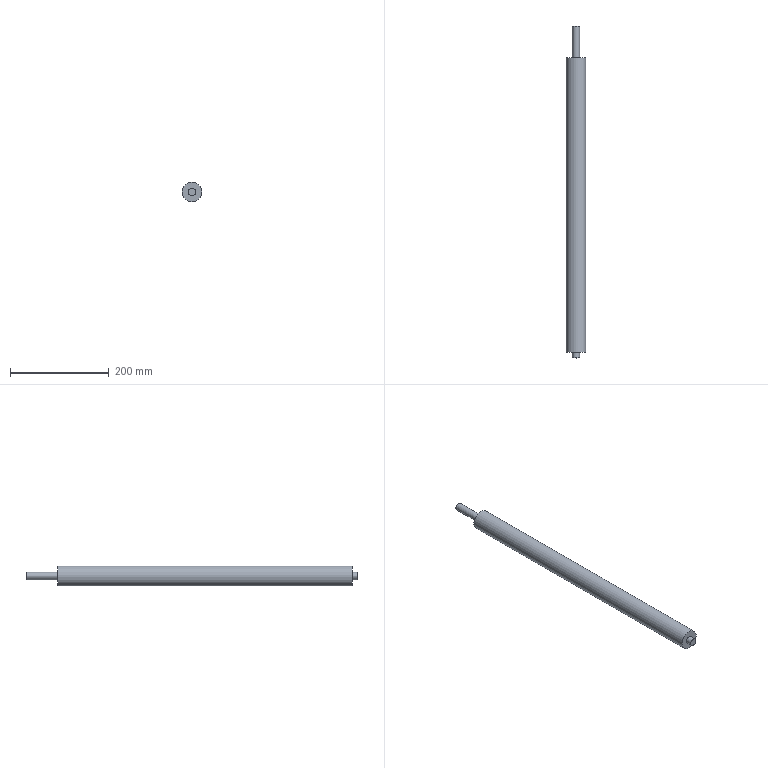Part | STEP file | songzhizhou | 1 solid | 7 faces | box 40 x 672 x 40 mm | volume 762386 mm3 | plane 4 | cylinder 3 | commonest cylinder face diameters 15 x2 40 x1
STEP:
#1=CARTESIAN_POINT('',(0.,0.,0.));
#2=DIRECTION('',(0.,0.,1.));
#3=DIRECTION('',(1.,0.,0.));
#4=AXIS2_PLACEMENT_3D('',#1,#2,#3);
#5=CARTESIAN_POINT('',(0.,12.,7.5));
#6=VERTEX_POINT('',#5);
#7=CARTESIAN_POINT('',(0.,12.,0.));
#8=DIRECTION('',(0.,1.,0.));
#9=DIRECTION('',(0.,0.,1.));
#10=AXIS2_PLACEMENT_3D('',#7,#8,#9);
#11=CIRCLE('',#10,7.5);
#12=CARTESIAN_POINT('',(0.,12.,0.));
#13=DIRECTION('',(0.,-1.,0.));
#14=DIRECTION('',(0.,0.,-1.));
#15=AXIS2_PLACEMENT_3D('',#12,#13,#14);
#16=CYLINDRICAL_SURFACE('',#15,7.5);
#17=CARTESIAN_POINT('',(9.425,0.));
#18=DIRECTION('',(-1.,0.));
#19=VECTOR('',#18,1.);
#20=LINE('',#17,#19);
#21=(GEOMETRIC_REPRESENTATION_CONTEXT(2)PARAMETRIC_REPRESENTATION_CONTEXT()REPRESENTATION_CONTEXT('',''));
#22=DEFINITIONAL_REPRESENTATION('',(#20),#21);
#23=PCURVE('',#16,#22);
#24=CARTESIAN_POINT('',(0.,12.,0.));
#25=DIRECTION('',(0.,1.,0.));
#26=DIRECTION('',(0.,0.,1.));
#27=AXIS2_PLACEMENT_3D('',#24,#25,#26);
#28=PLANE('',#27);
#29=CARTESIAN_POINT('',(0.,0.));
#30=DIRECTION('',(1.,0.));
#31=AXIS2_PLACEMENT_2D('',#29,#30);
#32=CIRCLE('',#31,7.5);
#33=(GEOMETRIC_REPRESENTATION_CONTEXT(2)PARAMETRIC_REPRESENTATION_CONTEXT()REPRESENTATION_CONTEXT('',''));
#34=DEFINITIONAL_REPRESENTATION('',(#32),#33);
#35=PCURVE('',#28,#34);
#36=SURFACE_CURVE('',#11,(#23,#35),.PCURVE_S1.);
#37=EDGE_CURVE('',#6,#6,#36,.T.);
#38=ORIENTED_EDGE('',*,*,#37,.F.);
#39=CARTESIAN_POINT('',(0.,0.,7.5));
#40=VERTEX_POINT('',#39);
#41=CARTESIAN_POINT('',(0.,12.,7.5));
#42=CARTESIAN_POINT('',(0.,0.,7.5));
#43=B_SPLINE_CURVE_WITH_KNOTS('',1,(#41,#42),.UNSPECIFIED.,.F.,.F.,(2,2),(0.,12.),.PIECEWISE_BEZIER_KNOTS.);
#44=CARTESIAN_POINT('',(9.425,0.));
#45=DIRECTION('',(0.,1.));
#46=VECTOR('',#45,1.);
#47=LINE('',#44,#46);
#48=(GEOMETRIC_REPRESENTATION_CONTEXT(2)PARAMETRIC_REPRESENTATION_CONTEXT()REPRESENTATION_CONTEXT('',''));
#49=DEFINITIONAL_REPRESENTATION('',(#47),#48);
#50=PCURVE('',#16,#49);
#51=CARTESIAN_POINT('',(3.142,0.));
#52=DIRECTION('',(0.,1.));
#53=VECTOR('',#52,1.);
#54=LINE('',#51,#53);
#55=(GEOMETRIC_REPRESENTATION_CONTEXT(2)PARAMETRIC_REPRESENTATION_CONTEXT()REPRESENTATION_CONTEXT('',''));
#56=DEFINITIONAL_REPRESENTATION('',(#54),#55);
#57=PCURVE('',#16,#56);
#58=SEAM_CURVE('',#43,(#50,#57),.PCURVE_S1.);
#59=EDGE_CURVE('',#6,#40,#58,.T.);
#60=ORIENTED_EDGE('',*,*,#59,.T.);
#61=CARTESIAN_POINT('',(0.,0.,0.));
#62=DIRECTION('',(0.,1.,0.));
#63=DIRECTION('',(0.,0.,1.));
#64=AXIS2_PLACEMENT_3D('',#61,#62,#63);
#65=CIRCLE('',#64,7.5);
#66=CARTESIAN_POINT('',(9.425,12.));
#67=DIRECTION('',(-1.,0.));
#68=VECTOR('',#67,1.);
#69=LINE('',#66,#68);
#70=(GEOMETRIC_REPRESENTATION_CONTEXT(2)PARAMETRIC_REPRESENTATION_CONTEXT()REPRESENTATION_CONTEXT('',''));
#71=DEFINITIONAL_REPRESENTATION('',(#69),#70);
#72=PCURVE('',#16,#71);
#73=CARTESIAN_POINT('',(0.,0.,0.));
#74=DIRECTION('',(0.,1.,0.));
#75=DIRECTION('',(0.,0.,1.));
#76=AXIS2_PLACEMENT_3D('',#73,#74,#75);
#77=PLANE('',#76);
#78=CARTESIAN_POINT('',(0.,0.));
#79=DIRECTION('',(1.,0.));
#80=AXIS2_PLACEMENT_2D('',#78,#79);
#81=CIRCLE('',#80,7.5);
#82=(GEOMETRIC_REPRESENTATION_CONTEXT(2)PARAMETRIC_REPRESENTATION_CONTEXT()REPRESENTATION_CONTEXT('',''));
#83=DEFINITIONAL_REPRESENTATION('',(#81),#82);
#84=PCURVE('',#77,#83);
#85=SURFACE_CURVE('',#65,(#72,#84),.PCURVE_S1.);
#86=EDGE_CURVE('',#40,#40,#85,.T.);
#87=ORIENTED_EDGE('',*,*,#86,.T.);
#88=ORIENTED_EDGE('',*,*,#59,.F.);
#89=EDGE_LOOP('',(#38,#60,#87,#88));
#90=FACE_BOUND('',#89,.T.);
#91=ADVANCED_FACE('',(#90),#16,.T.);
#92=ORIENTED_EDGE('',*,*,#86,.F.);
#93=EDGE_LOOP('',(#92));
#94=FACE_BOUND('',#93,.T.);
#95=ADVANCED_FACE('',(#94),#77,.F.);
#96=CARTESIAN_POINT('',(0.,608.,20.));
#97=VERTEX_POINT('',#96);
#98=CARTESIAN_POINT('',(0.,608.,0.));
#99=DIRECTION('',(0.,1.,0.));
#100=DIRECTION('',(0.,0.,1.));
#101=AXIS2_PLACEMENT_3D('',#98,#99,#100);
#102=CIRCLE('',#101,20.);
#103=CARTESIAN_POINT('',(0.,608.,0.));
#104=DIRECTION('',(0.,-1.,0.));
#105=DIRECTION('',(0.,0.,-1.));
#106=AXIS2_PLACEMENT_3D('',#103,#104,#105);
#107=CYLINDRICAL_SURFACE('',#106,20.);
#108=CARTESIAN_POINT('',(9.425,0.));
#109=DIRECTION('',(-1.,0.));
#110=VECTOR('',#109,1.);
#111=LINE('',#108,#110);
#112=(GEOMETRIC_REPRESENTATION_CONTEXT(2)PARAMETRIC_REPRESENTATION_CONTEXT()REPRESENTATION_CONTEXT('',''));
#113=DEFINITIONAL_REPRESENTATION('',(#111),#112);
#114=PCURVE('',#107,#113);
#115=CARTESIAN_POINT('',(0.,608.,0.));
#116=DIRECTION('',(0.,1.,0.));
#117=DIRECTION('',(0.,0.,1.));
#118=AXIS2_PLACEMENT_3D('',#115,#116,#117);
#119=PLANE('',#118);
#120=CARTESIAN_POINT('',(0.,0.));
#121=DIRECTION('',(1.,0.));
#122=AXIS2_PLACEMENT_2D('',#120,#121);
#123=CIRCLE('',#122,20.);
#124=(GEOMETRIC_REPRESENTATION_CONTEXT(2)PARAMETRIC_REPRESENTATION_CONTEXT()REPRESENTATION_CONTEXT('',''));
#125=DEFINITIONAL_REPRESENTATION('',(#123),#124);
#126=PCURVE('',#119,#125);
#127=SURFACE_CURVE('',#102,(#114,#126),.PCURVE_S1.);
#128=EDGE_CURVE('',#97,#97,#127,.T.);
#129=ORIENTED_EDGE('',*,*,#128,.F.);
#130=CARTESIAN_POINT('',(0.,12.,20.));
#131=VERTEX_POINT('',#130);
#132=CARTESIAN_POINT('',(0.,608.,20.));
#133=CARTESIAN_POINT('',(0.,12.,20.));
#134=B_SPLINE_CURVE_WITH_KNOTS('',1,(#132,#133),.UNSPECIFIED.,.F.,.F.,(2,2),(0.,596.),.PIECEWISE_BEZIER_KNOTS.);
#135=CARTESIAN_POINT('',(9.425,0.));
#136=DIRECTION('',(0.,1.));
#137=VECTOR('',#136,1.);
#138=LINE('',#135,#137);
#139=(GEOMETRIC_REPRESENTATION_CONTEXT(2)PARAMETRIC_REPRESENTATION_CONTEXT()REPRESENTATION_CONTEXT('',''));
#140=DEFINITIONAL_REPRESENTATION('',(#138),#139);
#141=PCURVE('',#107,#140);
#142=CARTESIAN_POINT('',(3.142,0.));
#143=DIRECTION('',(0.,1.));
#144=VECTOR('',#143,1.);
#145=LINE('',#142,#144);
#146=(GEOMETRIC_REPRESENTATION_CONTEXT(2)PARAMETRIC_REPRESENTATION_CONTEXT()REPRESENTATION_CONTEXT('',''));
#147=DEFINITIONAL_REPRESENTATION('',(#145),#146);
#148=PCURVE('',#107,#147);
#149=SEAM_CURVE('',#134,(#141,#148),.PCURVE_S1.);
#150=EDGE_CURVE('',#97,#131,#149,.T.);
#151=ORIENTED_EDGE('',*,*,#150,.T.);
#152=CARTESIAN_POINT('',(0.,12.,0.));
#153=DIRECTION('',(0.,1.,0.));
#154=DIRECTION('',(0.,0.,1.));
#155=AXIS2_PLACEMENT_3D('',#152,#153,#154);
#156=CIRCLE('',#155,20.);
#157=CARTESIAN_POINT('',(9.425,596.));
#158=DIRECTION('',(-1.,0.));
#159=VECTOR('',#158,1.);
#160=LINE('',#157,#159);
#161=(GEOMETRIC_REPRESENTATION_CONTEXT(2)PARAMETRIC_REPRESENTATION_CONTEXT()REPRESENTATION_CONTEXT('',''));
#162=DEFINITIONAL_REPRESENTATION('',(#160),#161);
#163=PCURVE('',#107,#162);
#164=CARTESIAN_POINT('',(0.,0.));
#165=DIRECTION('',(1.,0.));
#166=AXIS2_PLACEMENT_2D('',#164,#165);
#167=CIRCLE('',#166,20.);
#168=(GEOMETRIC_REPRESENTATION_CONTEXT(2)PARAMETRIC_REPRESENTATION_CONTEXT()REPRESENTATION_CONTEXT('',''));
#169=DEFINITIONAL_REPRESENTATION('',(#167),#168);
#170=PCURVE('',#28,#169);
#171=SURFACE_CURVE('',#156,(#163,#170),.PCURVE_S1.);
#172=EDGE_CURVE('',#131,#131,#171,.T.);
#173=ORIENTED_EDGE('',*,*,#172,.T.);
#174=ORIENTED_EDGE('',*,*,#150,.F.);
#175=EDGE_LOOP('',(#129,#151,#173,#174));
#176=FACE_BOUND('',#175,.T.);
#177=ADVANCED_FACE('',(#176),#107,.T.);
#178=CARTESIAN_POINT('',(0.,608.,7.5));
#179=VERTEX_POINT('',#178);
#180=CARTESIAN_POINT('',(0.,608.,0.));
#181=DIRECTION('',(0.,1.,0.));
#182=DIRECTION('',(0.,0.,1.));
#183=AXIS2_PLACEMENT_3D('',#180,#181,#182);
#184=CIRCLE('',#183,7.5);
#185=CARTESIAN_POINT('',(0.,0.));
#186=DIRECTION('',(1.,0.));
#187=AXIS2_PLACEMENT_2D('',#185,#186);
#188=CIRCLE('',#187,7.5);
#189=(GEOMETRIC_REPRESENTATION_CONTEXT(2)PARAMETRIC_REPRESENTATION_CONTEXT()REPRESENTATION_CONTEXT('',''));
#190=DEFINITIONAL_REPRESENTATION('',(#188),#189);
#191=PCURVE('',#119,#190);
#192=CARTESIAN_POINT('',(0.,672.,0.));
#193=DIRECTION('',(0.,-1.,0.));
#194=DIRECTION('',(0.,0.,-1.));
#195=AXIS2_PLACEMENT_3D('',#192,#193,#194);
#196=CYLINDRICAL_SURFACE('',#195,7.5);
#197=CARTESIAN_POINT('',(9.425,64.));
#198=DIRECTION('',(-1.,0.));
#199=VECTOR('',#198,1.);
#200=LINE('',#197,#199);
#201=(GEOMETRIC_REPRESENTATION_CONTEXT(2)PARAMETRIC_REPRESENTATION_CONTEXT()REPRESENTATION_CONTEXT('',''));
#202=DEFINITIONAL_REPRESENTATION('',(#200),#201);
#203=PCURVE('',#196,#202);
#204=SURFACE_CURVE('',#184,(#191,#203),.PCURVE_S1.);
#205=EDGE_CURVE('',#179,#179,#204,.T.);
#206=ORIENTED_EDGE('',*,*,#205,.F.);
#207=EDGE_LOOP('',(#206));
#208=FACE_BOUND('',#207,.T.);
#209=ORIENTED_EDGE('',*,*,#128,.T.);
#210=EDGE_LOOP('',(#209));
#211=FACE_BOUND('',#210,.T.);
#212=ADVANCED_FACE('',(#208,#211),#119,.T.);
#213=ORIENTED_EDGE('',*,*,#37,.T.);
#214=EDGE_LOOP('',(#213));
#215=FACE_BOUND('',#214,.T.);
#216=ORIENTED_EDGE('',*,*,#172,.F.);
#217=EDGE_LOOP('',(#216));
#218=FACE_BOUND('',#217,.T.);
#219=ADVANCED_FACE('',(#215,#218),#28,.F.);
#220=CARTESIAN_POINT('',(0.,672.,7.5));
#221=VERTEX_POINT('',#220);
#222=CARTESIAN_POINT('',(0.,672.,0.));
#223=DIRECTION('',(0.,1.,0.));
#224=DIRECTION('',(0.,0.,1.));
#225=AXIS2_PLACEMENT_3D('',#222,#223,#224);
#226=CIRCLE('',#225,7.5);
#227=CARTESIAN_POINT('',(9.425,0.));
#228=DIRECTION('',(-1.,0.));
#229=VECTOR('',#228,1.);
#230=LINE('',#227,#229);
#231=(GEOMETRIC_REPRESENTATION_CONTEXT(2)PARAMETRIC_REPRESENTATION_CONTEXT()REPRESENTATION_CONTEXT('',''));
#232=DEFINITIONAL_REPRESENTATION('',(#230),#231);
#233=PCURVE('',#196,#232);
#234=CARTESIAN_POINT('',(0.,672.,0.));
#235=DIRECTION('',(0.,1.,0.));
#236=DIRECTION('',(0.,0.,1.));
#237=AXIS2_PLACEMENT_3D('',#234,#235,#236);
#238=PLANE('',#237);
#239=CARTESIAN_POINT('',(0.,0.));
#240=DIRECTION('',(1.,0.));
#241=AXIS2_PLACEMENT_2D('',#239,#240);
#242=CIRCLE('',#241,7.5);
#243=(GEOMETRIC_REPRESENTATION_CONTEXT(2)PARAMETRIC_REPRESENTATION_CONTEXT()REPRESENTATION_CONTEXT('',''));
#244=DEFINITIONAL_REPRESENTATION('',(#242),#243);
#245=PCURVE('',#238,#244);
#246=SURFACE_CURVE('',#226,(#233,#245),.PCURVE_S1.);
#247=EDGE_CURVE('',#221,#221,#246,.T.);
#248=ORIENTED_EDGE('',*,*,#247,.F.);
#249=CARTESIAN_POINT('',(0.,672.,7.5));
#250=CARTESIAN_POINT('',(0.,608.,7.5));
#251=B_SPLINE_CURVE_WITH_KNOTS('',1,(#249,#250),.UNSPECIFIED.,.F.,.F.,(2,2),(0.,64.),.PIECEWISE_BEZIER_KNOTS.);
#252=CARTESIAN_POINT('',(9.425,0.));
#253=DIRECTION('',(0.,1.));
#254=VECTOR('',#253,1.);
#255=LINE('',#252,#254);
#256=(GEOMETRIC_REPRESENTATION_CONTEXT(2)PARAMETRIC_REPRESENTATION_CONTEXT()REPRESENTATION_CONTEXT('',''));
#257=DEFINITIONAL_REPRESENTATION('',(#255),#256);
#258=PCURVE('',#196,#257);
#259=CARTESIAN_POINT('',(3.142,0.));
#260=DIRECTION('',(0.,1.));
#261=VECTOR('',#260,1.);
#262=LINE('',#259,#261);
#263=(GEOMETRIC_REPRESENTATION_CONTEXT(2)PARAMETRIC_REPRESENTATION_CONTEXT()REPRESENTATION_CONTEXT('',''));
#264=DEFINITIONAL_REPRESENTATION('',(#262),#263);
#265=PCURVE('',#196,#264);
#266=SEAM_CURVE('',#251,(#258,#265),.PCURVE_S1.);
#267=EDGE_CURVE('',#221,#179,#266,.T.);
#268=ORIENTED_EDGE('',*,*,#267,.T.);
#269=ORIENTED_EDGE('',*,*,#205,.T.);
#270=ORIENTED_EDGE('',*,*,#267,.F.);
#271=EDGE_LOOP('',(#248,#268,#269,#270));
#272=FACE_BOUND('',#271,.T.);
#273=ADVANCED_FACE('',(#272),#196,.T.);
#274=ORIENTED_EDGE('',*,*,#247,.T.);
#275=EDGE_LOOP('',(#274));
#276=FACE_BOUND('',#275,.T.);
#277=ADVANCED_FACE('',(#276),#238,.T.);
#278=CLOSED_SHELL('',(#91,#95,#177,#212,#219,#273,#277));
#279=MANIFOLD_SOLID_BREP('',#278);
#280=(LENGTH_UNIT()NAMED_UNIT(*)SI_UNIT(.MILLI.,.METRE.));
#281=UNCERTAINTY_MEASURE_WITH_UNIT(LENGTH_MEASURE(0.00001),#280,'','');
#282=(NAMED_UNIT(*)PLANE_ANGLE_UNIT()SI_UNIT($,.RADIAN.));
#283=(NAMED_UNIT(*)SI_UNIT($,.STERADIAN.)SOLID_ANGLE_UNIT());
#284=(GEOMETRIC_REPRESENTATION_CONTEXT(3)GLOBAL_UNCERTAINTY_ASSIGNED_CONTEXT((#281))GLOBAL_UNIT_ASSIGNED_CONTEXT((#280,#282,#283))REPRESENTATION_CONTEXT('',''));
#285=ADVANCED_BREP_SHAPE_REPRESENTATION('',(#4,#279),#284);